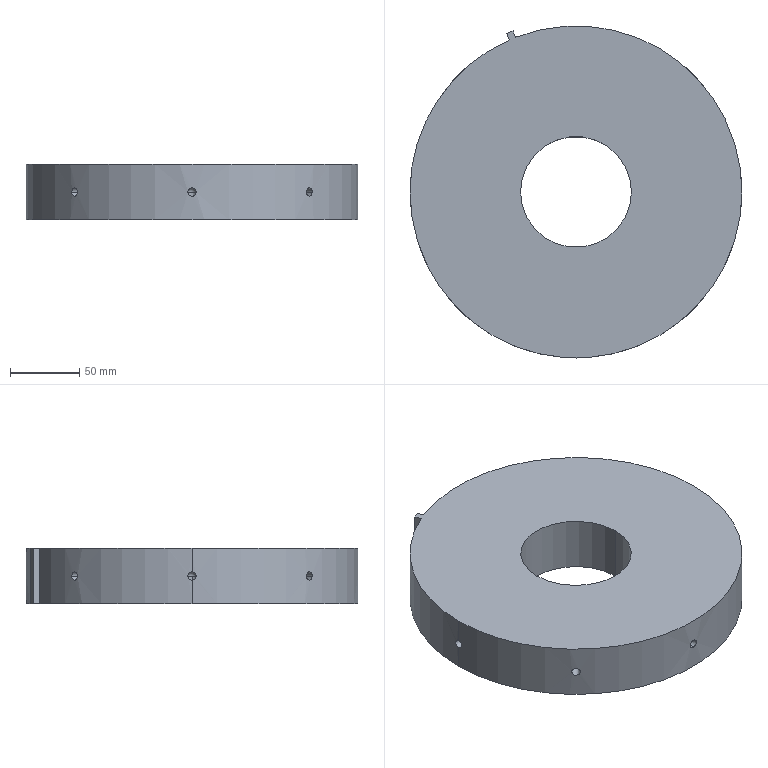Part | SolidWorks | features ICE 4, CirPattern 1, Extrusion 1, RevCut 1 | 1 solid | 74 faces | box 240 x 240 x 40 mm | volume 1593754 mm3 | cylinder 53 | plane 13 | sphere 8 | commonest cylinder face diameters 6 x32 5.31 x16 240 x3 80.06 x2